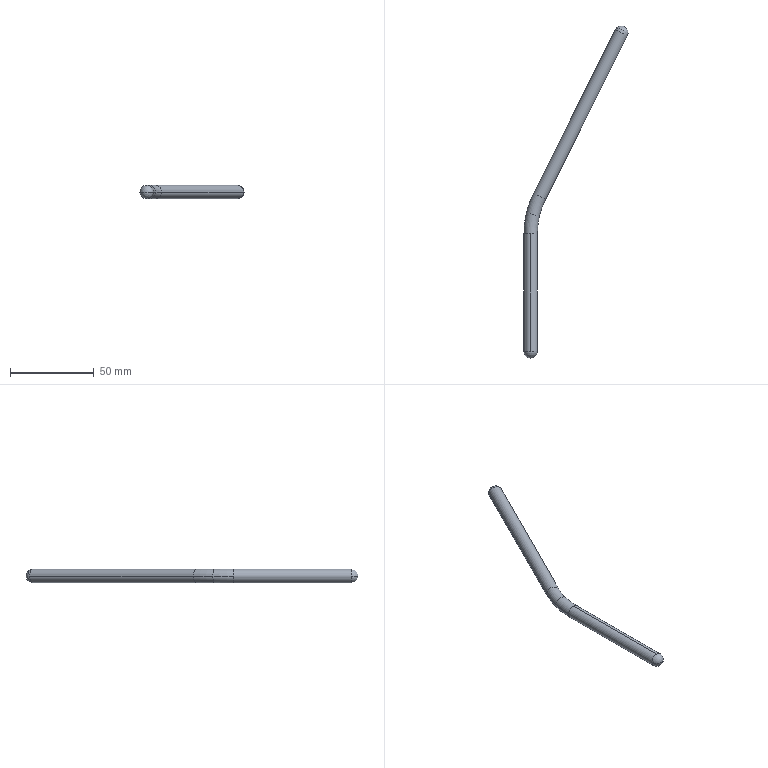Part | Creo | 1 solid | 12 faces | box 62.122 x 198.229 x 8 mm | volume 10451 mm3 | cylinder 4 | sphere 4 | torus 4 | commonest cylinder face diameters 8 x4
STEP:
#1=CARTESIAN_POINT('',(-56.384,-202.75,38.161));
#2=VERTEX_POINT('',#1);
#3=CARTESIAN_POINT('',(-60.384,-202.75,42.161));
#4=VERTEX_POINT('',#3);
#5=CARTESIAN_POINT('',(-60.384,-202.75,38.161));
#6=DIRECTION('',(0.,-1.,0.));
#7=DIRECTION('',(1.,0.,0.));
#8=AXIS2_PLACEMENT_3D('',#5,#6,#7);
#9=CIRCLE('',#8,4.);
#10=EDGE_CURVE('',#2,#4,#9,.T.);
#11=ORIENTED_EDGE('',*,*,#10,.T.);
#12=CARTESIAN_POINT('',(-60.384,-132.555,42.161));
#13=VERTEX_POINT('',#12);
#14=CARTESIAN_POINT('',(-60.384,-132.555,42.161));
#15=DIRECTION('',(0.,-1.,0.));
#16=VECTOR('',#15,70.195);
#17=LINE('',#14,#16);
#18=EDGE_CURVE('',#13,#4,#17,.T.);
#19=ORIENTED_EDGE('',*,*,#18,.F.);
#20=CARTESIAN_POINT('',(-56.384,-132.555,38.161));
#21=VERTEX_POINT('',#20);
#22=CARTESIAN_POINT('',(-60.384,-132.555,38.161));
#23=DIRECTION('',(0.,1.,0.));
#24=DIRECTION('',(0.,0.,1.));
#25=AXIS2_PLACEMENT_3D('',#22,#23,#24);
#26=CIRCLE('',#25,4.);
#27=EDGE_CURVE('',#13,#21,#26,.T.);
#28=ORIENTED_EDGE('',*,*,#27,.T.);
#29=CARTESIAN_POINT('',(-60.384,-132.555,34.161));
#30=VERTEX_POINT('',#29);
#31=CARTESIAN_POINT('',(-60.384,-132.555,38.161));
#32=DIRECTION('',(0.,1.,0.));
#33=DIRECTION('',(1.,0.,0.));
#34=AXIS2_PLACEMENT_3D('',#31,#32,#33);
#35=CIRCLE('',#34,4.);
#36=EDGE_CURVE('',#21,#30,#35,.T.);
#37=ORIENTED_EDGE('',*,*,#36,.T.);
#38=CARTESIAN_POINT('',(-60.384,-202.75,34.161));
#39=VERTEX_POINT('',#38);
#40=CARTESIAN_POINT('',(-60.384,-132.555,34.161));
#41=DIRECTION('',(0.,-1.,0.));
#42=VECTOR('',#41,70.195);
#43=LINE('',#40,#42);
#44=EDGE_CURVE('',#30,#39,#43,.T.);
#45=ORIENTED_EDGE('',*,*,#44,.T.);
#46=CARTESIAN_POINT('',(-60.384,-202.75,38.161));
#47=DIRECTION('',(0.,-1.,0.));
#48=DIRECTION('',(0.,0.,-1.));
#49=AXIS2_PLACEMENT_3D('',#46,#47,#48);
#50=CIRCLE('',#49,4.);
#51=EDGE_CURVE('',#39,#2,#50,.T.);
#52=ORIENTED_EDGE('',*,*,#51,.T.);
#53=EDGE_LOOP('',(#11,#19,#28,#37,#45,#52));
#54=FACE_OUTER_BOUND('',#53,.F.);
#55=CARTESIAN_POINT('',(-60.384,-132.555,38.161));
#56=DIRECTION('',(0.,-1.,0.));
#57=DIRECTION('',(0.,0.,-1.));
#58=AXIS2_PLACEMENT_3D('',#55,#56,#57);
#59=CYLINDRICAL_SURFACE('',#58,4.);
#60=ADVANCED_FACE('',(#54),#59,.T.);
#61=CARTESIAN_POINT('',(-64.384,-202.75,38.161));
#62=VERTEX_POINT('',#61);
#63=CARTESIAN_POINT('',(-60.384,-202.75,38.161));
#64=DIRECTION('',(0.,-1.,0.));
#65=DIRECTION('',(0.,0.,1.));
#66=AXIS2_PLACEMENT_3D('',#63,#64,#65);
#67=CIRCLE('',#66,4.);
#68=EDGE_CURVE('',#4,#62,#67,.T.);
#69=ORIENTED_EDGE('',*,*,#68,.F.);
#70=ORIENTED_EDGE('',*,*,#10,.F.);
#71=CARTESIAN_POINT('',(-60.384,-206.75,38.161));
#72=VERTEX_POINT('',#71);
#73=CARTESIAN_POINT('',(-60.384,-202.75,38.161));
#74=DIRECTION('',(0.,0.,1.));
#75=DIRECTION('',(0.,-1.,0.));
#76=AXIS2_PLACEMENT_3D('',#73,#74,#75);
#77=CIRCLE('',#76,4.);
#78=EDGE_CURVE('',#72,#2,#77,.T.);
#79=ORIENTED_EDGE('',*,*,#78,.F.);
#80=CARTESIAN_POINT('',(-60.384,-202.75,38.161));
#81=DIRECTION('',(0.,0.,-1.));
#82=DIRECTION('',(0.,-1.,0.));
#83=AXIS2_PLACEMENT_3D('',#80,#81,#82);
#84=CIRCLE('',#83,4.);
#85=EDGE_CURVE('',#72,#62,#84,.T.);
#86=ORIENTED_EDGE('',*,*,#85,.T.);
#87=EDGE_LOOP('',(#69,#70,#79,#86));
#88=FACE_OUTER_BOUND('',#87,.F.);
#89=CARTESIAN_POINT('',(-60.384,-202.75,38.161));
#90=DIRECTION('',(0.,1.,0.));
#91=DIRECTION('',(1.,0.,0.));
#92=AXIS2_PLACEMENT_3D('',#89,#90,#91);
#93=SPHERICAL_SURFACE('',#92,4.);
#94=ADVANCED_FACE('',(#88),#93,.T.);
#95=CARTESIAN_POINT('',(-60.384,-202.75,38.161));
#96=DIRECTION('',(0.,-1.,0.));
#97=DIRECTION('',(-1.,0.,0.));
#98=AXIS2_PLACEMENT_3D('',#95,#96,#97);
#99=CIRCLE('',#98,4.);
#100=EDGE_CURVE('',#62,#39,#99,.T.);
#101=ORIENTED_EDGE('',*,*,#100,.T.);
#102=ORIENTED_EDGE('',*,*,#44,.F.);
#103=CARTESIAN_POINT('',(-64.384,-132.555,38.161));
#104=VERTEX_POINT('',#103);
#105=CARTESIAN_POINT('',(-60.384,-132.555,38.161));
#106=DIRECTION('',(0.,1.,0.));
#107=DIRECTION('',(0.,0.,-1.));
#108=AXIS2_PLACEMENT_3D('',#105,#106,#107);
#109=CIRCLE('',#108,4.);
#110=EDGE_CURVE('',#30,#104,#109,.T.);
#111=ORIENTED_EDGE('',*,*,#110,.T.);
#112=CARTESIAN_POINT('',(-60.384,-132.555,38.161));
#113=DIRECTION('',(0.,1.,0.));
#114=DIRECTION('',(-1.,0.,0.));
#115=AXIS2_PLACEMENT_3D('',#112,#113,#114);
#116=CIRCLE('',#115,4.);
#117=EDGE_CURVE('',#104,#13,#116,.T.);
#118=ORIENTED_EDGE('',*,*,#117,.T.);
#119=ORIENTED_EDGE('',*,*,#18,.T.);
#120=ORIENTED_EDGE('',*,*,#68,.T.);
#121=EDGE_LOOP('',(#101,#102,#111,#118,#119,#120));
#122=FACE_OUTER_BOUND('',#121,.F.);
#123=CARTESIAN_POINT('',(-60.384,-132.555,38.161));
#124=DIRECTION('',(0.,-1.,0.));
#125=DIRECTION('',(0.,0.,-1.));
#126=AXIS2_PLACEMENT_3D('',#123,#124,#125);
#127=CYLINDRICAL_SURFACE('',#126,4.);
#128=ADVANCED_FACE('',(#122),#127,.T.);
#129=ORIENTED_EDGE('',*,*,#100,.F.);
#130=ORIENTED_EDGE('',*,*,#85,.F.);
#131=ORIENTED_EDGE('',*,*,#78,.T.);
#132=ORIENTED_EDGE('',*,*,#51,.F.);
#133=EDGE_LOOP('',(#129,#130,#131,#132));
#134=FACE_OUTER_BOUND('',#133,.F.);
#135=CARTESIAN_POINT('',(-60.384,-202.75,38.161));
#136=DIRECTION('',(0.,1.,0.));
#137=DIRECTION('',(1.,0.,0.));
#138=AXIS2_PLACEMENT_3D('',#135,#136,#137);
#139=SPHERICAL_SURFACE('',#138,4.);
#140=ADVANCED_FACE('',(#134),#139,.T.);
#141=ORIENTED_EDGE('',*,*,#36,.F.);
#142=CARTESIAN_POINT('',(-55.153,-121.985,38.161));
#143=VERTEX_POINT('',#142);
#144=CARTESIAN_POINT('',(-10.384,-132.555,38.161));
#145=DIRECTION('',(0.,0.,1.));
#146=DIRECTION('',(-0.9732,0.2298,0.));
#147=AXIS2_PLACEMENT_3D('',#144,#145,#146);
#148=CIRCLE('',#147,46.);
#149=EDGE_CURVE('',#143,#21,#148,.T.);
#150=ORIENTED_EDGE('',*,*,#149,.F.);
#151=CARTESIAN_POINT('',(-62.939,-120.147,38.161));
#152=VERTEX_POINT('',#151);
#153=CARTESIAN_POINT('',(-59.046,-121.066,38.161));
#154=DIRECTION('',(0.2298,0.9732,0.));
#155=DIRECTION('',(0.9732,-0.2298,0.));
#156=AXIS2_PLACEMENT_3D('',#153,#154,#155);
#157=CIRCLE('',#156,4.);
#158=EDGE_CURVE('',#143,#152,#157,.T.);
#159=ORIENTED_EDGE('',*,*,#158,.T.);
#160=CARTESIAN_POINT('',(-10.384,-132.555,38.161));
#161=DIRECTION('',(0.,0.,1.));
#162=DIRECTION('',(-0.9732,0.2298,0.));
#163=AXIS2_PLACEMENT_3D('',#160,#161,#162);
#164=CIRCLE('',#163,54.);
#165=EDGE_CURVE('',#152,#104,#164,.T.);
#166=ORIENTED_EDGE('',*,*,#165,.T.);
#167=ORIENTED_EDGE('',*,*,#110,.F.);
#168=EDGE_LOOP('',(#141,#150,#159,#166,#167));
#169=FACE_OUTER_BOUND('',#168,.F.);
#170=CARTESIAN_POINT('',(-10.384,-132.555,38.161));
#171=DIRECTION('',(0.,0.,1.));
#172=DIRECTION('',(1.,0.,0.));
#173=AXIS2_PLACEMENT_3D('',#170,#171,#172);
#174=TOROIDAL_SURFACE('',#173,50.,4.);
#175=ADVANCED_FACE('',(#169),#174,.T.);
#176=ORIENTED_EDGE('',*,*,#117,.F.);
#177=ORIENTED_EDGE('',*,*,#165,.F.);
#178=CARTESIAN_POINT('',(-59.046,-121.066,38.161));
#179=DIRECTION('',(0.2298,0.9732,0.));
#180=DIRECTION('',(-0.9732,0.2298,0.));
#181=AXIS2_PLACEMENT_3D('',#178,#179,#180);
#182=CIRCLE('',#181,4.);
#183=EDGE_CURVE('',#152,#143,#182,.T.);
#184=ORIENTED_EDGE('',*,*,#183,.T.);
#185=ORIENTED_EDGE('',*,*,#149,.T.);
#186=ORIENTED_EDGE('',*,*,#27,.F.);
#187=EDGE_LOOP('',(#176,#177,#184,#185,#186));
#188=FACE_OUTER_BOUND('',#187,.F.);
#189=CARTESIAN_POINT('',(-10.384,-132.555,38.161));
#190=DIRECTION('',(0.,0.,1.));
#191=DIRECTION('',(1.,0.,0.));
#192=AXIS2_PLACEMENT_3D('',#189,#190,#191);
#193=TOROIDAL_SURFACE('',#192,50.,4.);
#194=ADVANCED_FACE('',(#188),#193,.T.);
#195=CARTESIAN_POINT('',(-51.526,-111.981,38.161));
#196=VERTEX_POINT('',#195);
#197=CARTESIAN_POINT('',(-58.681,-108.403,38.161));
#198=VERTEX_POINT('',#197);
#199=CARTESIAN_POINT('',(-55.104,-110.192,38.161));
#200=DIRECTION('',(-0.4473,-0.8944,0.));
#201=DIRECTION('',(0.8944,-0.4473,0.));
#202=AXIS2_PLACEMENT_3D('',#199,#200,#201);
#203=CIRCLE('',#202,4.);
#204=EDGE_CURVE('',#196,#198,#203,.T.);
#205=ORIENTED_EDGE('',*,*,#204,.F.);
#206=CARTESIAN_POINT('',(-10.384,-132.555,38.161));
#207=DIRECTION('',(0.,0.,1.));
#208=DIRECTION('',(-0.8944,0.4473,0.));
#209=AXIS2_PLACEMENT_3D('',#206,#207,#208);
#210=CIRCLE('',#209,46.);
#211=EDGE_CURVE('',#196,#143,#210,.T.);
#212=ORIENTED_EDGE('',*,*,#211,.T.);
#213=ORIENTED_EDGE('',*,*,#183,.F.);
#214=CARTESIAN_POINT('',(-10.384,-132.555,38.161));
#215=DIRECTION('',(0.,0.,1.));
#216=DIRECTION('',(-0.8944,0.4473,0.));
#217=AXIS2_PLACEMENT_3D('',#214,#215,#216);
#218=CIRCLE('',#217,54.);
#219=EDGE_CURVE('',#198,#152,#218,.T.);
#220=ORIENTED_EDGE('',*,*,#219,.F.);
#221=EDGE_LOOP('',(#205,#212,#213,#220));
#222=FACE_OUTER_BOUND('',#221,.F.);
#223=CARTESIAN_POINT('',(-10.384,-132.555,38.161));
#224=DIRECTION('',(0.,0.,1.));
#225=DIRECTION('',(1.,0.,0.));
#226=AXIS2_PLACEMENT_3D('',#223,#224,#225);
#227=TOROIDAL_SURFACE('',#226,50.,4.);
#228=ADVANCED_FACE('',(#222),#227,.T.);
#229=CARTESIAN_POINT('',(-9.839,-10.733,38.161));
#230=VERTEX_POINT('',#229);
#231=CARTESIAN_POINT('',(-2.684,-14.311,38.161));
#232=VERTEX_POINT('',#231);
#233=CARTESIAN_POINT('',(-6.262,-12.522,38.161));
#234=DIRECTION('',(0.4473,0.8944,0.));
#235=DIRECTION('',(-0.8944,0.4473,0.));
#236=AXIS2_PLACEMENT_3D('',#233,#234,#235);
#237=CIRCLE('',#236,4.);
#238=EDGE_CURVE('',#230,#232,#237,.T.);
#239=ORIENTED_EDGE('',*,*,#238,.T.);
#240=CARTESIAN_POINT('',(-51.526,-111.981,38.161));
#241=DIRECTION('',(0.4473,0.8944,0.));
#242=VECTOR('',#241,109.202);
#243=LINE('',#240,#242);
#244=EDGE_CURVE('',#196,#232,#243,.T.);
#245=ORIENTED_EDGE('',*,*,#244,.F.);
#246=ORIENTED_EDGE('',*,*,#204,.T.);
#247=CARTESIAN_POINT('',(-58.681,-108.403,38.161));
#248=DIRECTION('',(0.4473,0.8944,0.));
#249=VECTOR('',#248,109.202);
#250=LINE('',#247,#249);
#251=EDGE_CURVE('',#198,#230,#250,.T.);
#252=ORIENTED_EDGE('',*,*,#251,.T.);
#253=EDGE_LOOP('',(#239,#245,#246,#252));
#254=FACE_OUTER_BOUND('',#253,.F.);
#255=CARTESIAN_POINT('',(-55.104,-110.192,38.161));
#256=DIRECTION('',(0.4473,0.8944,0.));
#257=DIRECTION('',(-0.8944,0.4473,0.));
#258=AXIS2_PLACEMENT_3D('',#255,#256,#257);
#259=CYLINDRICAL_SURFACE('',#258,4.);
#260=ADVANCED_FACE('',(#254),#259,.T.);
#261=ORIENTED_EDGE('',*,*,#238,.F.);
#262=CARTESIAN_POINT('',(-6.262,-12.522,38.161));
#263=DIRECTION('',(-0.4,-0.8,0.4473));
#264=DIRECTION('',(0.8944,-0.4473,0.));
#265=AXIS2_PLACEMENT_3D('',#262,#263,#264);
#266=CIRCLE('',#265,4.);
#267=EDGE_CURVE('',#232,#230,#266,.T.);
#268=ORIENTED_EDGE('',*,*,#267,.F.);
#269=EDGE_LOOP('',(#261,#268));
#270=FACE_OUTER_BOUND('',#269,.F.);
#271=CARTESIAN_POINT('',(-6.262,-12.522,38.161));
#272=DIRECTION('',(-0.8944,0.4473,0.));
#273=DIRECTION('',(0.2,0.4,0.8944));
#274=AXIS2_PLACEMENT_3D('',#271,#272,#273);
#275=SPHERICAL_SURFACE('',#274,4.);
#276=ADVANCED_FACE('',(#270),#275,.T.);
#277=CARTESIAN_POINT('',(-6.262,-12.522,38.161));
#278=DIRECTION('',(0.4473,0.8944,0.));
#279=DIRECTION('',(0.8944,-0.4473,0.));
#280=AXIS2_PLACEMENT_3D('',#277,#278,#279);
#281=CIRCLE('',#280,4.);
#282=EDGE_CURVE('',#232,#230,#281,.T.);
#283=ORIENTED_EDGE('',*,*,#282,.F.);
#284=ORIENTED_EDGE('',*,*,#267,.T.);
#285=EDGE_LOOP('',(#283,#284));
#286=FACE_OUTER_BOUND('',#285,.F.);
#287=CARTESIAN_POINT('',(-6.262,-12.522,38.161));
#288=DIRECTION('',(-0.8944,0.4473,0.));
#289=DIRECTION('',(0.2,0.4,0.8944));
#290=AXIS2_PLACEMENT_3D('',#287,#288,#289);
#291=SPHERICAL_SURFACE('',#290,4.);
#292=ADVANCED_FACE('',(#286),#291,.T.);
#293=ORIENTED_EDGE('',*,*,#282,.T.);
#294=ORIENTED_EDGE('',*,*,#251,.F.);
#295=CARTESIAN_POINT('',(-55.104,-110.192,38.161));
#296=DIRECTION('',(-0.4473,-0.8944,0.));
#297=DIRECTION('',(-0.8944,0.4473,0.));
#298=AXIS2_PLACEMENT_3D('',#295,#296,#297);
#299=CIRCLE('',#298,4.);
#300=EDGE_CURVE('',#198,#196,#299,.T.);
#301=ORIENTED_EDGE('',*,*,#300,.T.);
#302=ORIENTED_EDGE('',*,*,#244,.T.);
#303=EDGE_LOOP('',(#293,#294,#301,#302));
#304=FACE_OUTER_BOUND('',#303,.F.);
#305=CARTESIAN_POINT('',(-55.104,-110.192,38.161));
#306=DIRECTION('',(0.4473,0.8944,0.));
#307=DIRECTION('',(-0.8944,0.4473,0.));
#308=AXIS2_PLACEMENT_3D('',#305,#306,#307);
#309=CYLINDRICAL_SURFACE('',#308,4.);
#310=ADVANCED_FACE('',(#304),#309,.T.);
#311=ORIENTED_EDGE('',*,*,#300,.F.);
#312=ORIENTED_EDGE('',*,*,#219,.T.);
#313=ORIENTED_EDGE('',*,*,#158,.F.);
#314=ORIENTED_EDGE('',*,*,#211,.F.);
#315=EDGE_LOOP('',(#311,#312,#313,#314));
#316=FACE_OUTER_BOUND('',#315,.F.);
#317=CARTESIAN_POINT('',(-10.384,-132.555,38.161));
#318=DIRECTION('',(0.,0.,1.));
#319=DIRECTION('',(1.,0.,0.));
#320=AXIS2_PLACEMENT_3D('',#317,#318,#319);
#321=TOROIDAL_SURFACE('',#320,50.,4.);
#322=ADVANCED_FACE('',(#316),#321,.T.);
#323=CLOSED_SHELL('',(#60,#94,#128,#140,#175,#194,#228,#260,#276,#292,#310,#322));
#324=MANIFOLD_SOLID_BREP('',#323);
#325=(LENGTH_UNIT()NAMED_UNIT(*)SI_UNIT(.MILLI.,.METRE.));
#326=UNCERTAINTY_MEASURE_WITH_UNIT(LENGTH_MEASURE(0.02079),#325,'','');
#327=(NAMED_UNIT(*)PLANE_ANGLE_UNIT()SI_UNIT($,.RADIAN.));
#328=PLANE_ANGLE_MEASURE_WITH_UNIT(PLANE_ANGLE_MEASURE(0.01745),#327);
#329=(CONVERSION_BASED_UNIT('DEGREE',#328)NAMED_UNIT(*)PLANE_ANGLE_UNIT());
#330=(NAMED_UNIT(*)SI_UNIT($,.STERADIAN.)SOLID_ANGLE_UNIT());
#331=(GEOMETRIC_REPRESENTATION_CONTEXT(3)GLOBAL_UNCERTAINTY_ASSIGNED_CONTEXT((#326))GLOBAL_UNIT_ASSIGNED_CONTEXT((#325,#329,#330))REPRESENTATION_CONTEXT('',''));
#332=ADVANCED_BREP_SHAPE_REPRESENTATION('',(#324),#331);